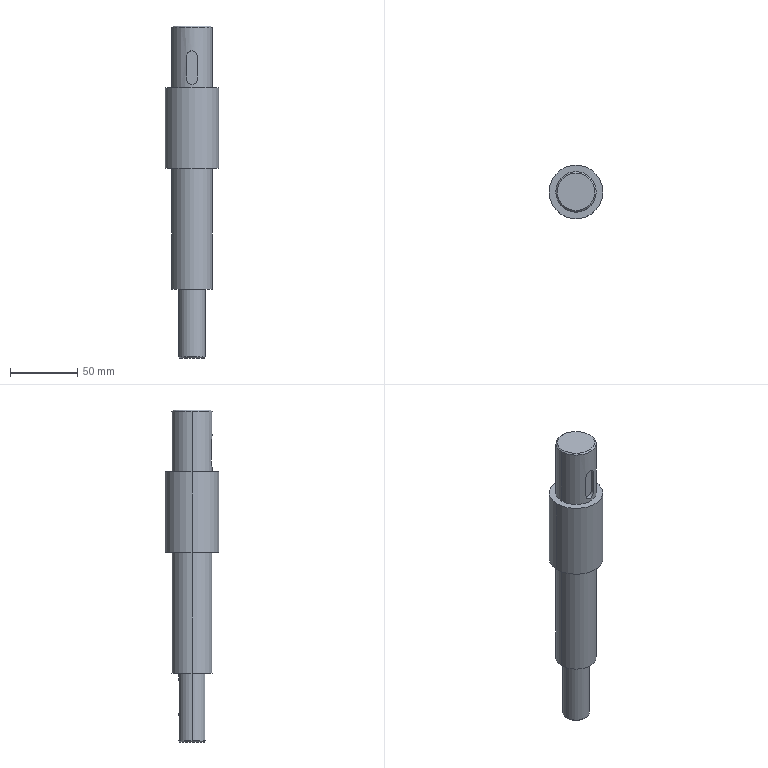Part | SolidWorks | features BaseBody 1 | 1 solid | 27 faces | box 40 x 40 x 247 mm | volume 186572 mm3 | cylinder 12 | plane 11 | cone 4 | commonest cylinder face diameters 30 x4 6 x2 8 x2 20 x2 40 x2
STEP:
#1=CARTESIAN_POINT('',(-9.,0.,0.));
#2=VERTEX_POINT('',#1);
#3=CARTESIAN_POINT('',(9.,0.,0.));
#4=VERTEX_POINT('',#3);
#5=CARTESIAN_POINT('',(0.,0.,0.));
#6=DIRECTION('',(0.,0.,1.));
#7=DIRECTION('',(-1.,0.,0.));
#8=AXIS2_PLACEMENT_3D('',#5,#6,#7);
#9=CIRCLE('',#8,9.);
#10=EDGE_CURVE('',#2,#4,#9,.T.);
#11=ORIENTED_EDGE('',*,*,#10,.T.);
#12=CARTESIAN_POINT('',(10.,0.,1.));
#13=VERTEX_POINT('',#12);
#14=CARTESIAN_POINT('',(9.5,0.,0.5));
#15=DIRECTION('',(0.7071,0.,0.7071));
#16=VECTOR('',#15,1000.);
#17=LINE('',#14,#16);
#18=EDGE_CURVE('',#4,#13,#17,.T.);
#19=ORIENTED_EDGE('',*,*,#18,.T.);
#20=CARTESIAN_POINT('',(-10.,0.,1.));
#21=VERTEX_POINT('',#20);
#22=CARTESIAN_POINT('',(0.,0.,1.));
#23=DIRECTION('',(0.,0.,-1.));
#24=DIRECTION('',(-1.,0.,0.));
#25=AXIS2_PLACEMENT_3D('',#22,#23,#24);
#26=CIRCLE('',#25,10.);
#27=EDGE_CURVE('',#13,#21,#26,.T.);
#28=ORIENTED_EDGE('',*,*,#27,.T.);
#29=CARTESIAN_POINT('',(-9.5,0.,0.5));
#30=DIRECTION('',(-0.7071,0.,0.7071));
#31=VECTOR('',#30,1000.);
#32=LINE('',#29,#31);
#33=EDGE_CURVE('',#2,#21,#32,.T.);
#34=ORIENTED_EDGE('',*,*,#33,.F.);
#35=EDGE_LOOP('',(#11,#19,#28,#34));
#36=FACE_OUTER_BOUND('',#35,.T.);
#37=CARTESIAN_POINT('',(0.,0.,0.5));
#38=DIRECTION('',(0.,0.,1.));
#39=DIRECTION('',(-1.,0.,0.));
#40=AXIS2_PLACEMENT_3D('',#37,#38,#39);
#41=CONICAL_SURFACE('',#40,9.5,0.7854);
#42=ADVANCED_FACE('',(#36),#41,.T.);
#43=CARTESIAN_POINT('',(-3.,9.539,44.5));
#44=VERTEX_POINT('',#43);
#45=CARTESIAN_POINT('',(-3.,9.539,22.5));
#46=VERTEX_POINT('',#45);
#47=CARTESIAN_POINT('',(-3.,9.539,0.));
#48=DIRECTION('',(0.,0.,-1.));
#49=VECTOR('',#48,1000.);
#50=LINE('',#47,#49);
#51=EDGE_CURVE('',#44,#46,#50,.T.);
#52=ORIENTED_EDGE('',*,*,#51,.T.);
#53=CARTESIAN_POINT('',(3.,9.539,22.5));
#54=VERTEX_POINT('',#53);
#55=CARTESIAN_POINT('',(-3.,9.539,22.5));
#56=CARTESIAN_POINT('',(-3.,9.539,22.301));
#57=CARTESIAN_POINT('',(-2.98,9.546,22.105));
#58=CARTESIAN_POINT('',(-2.904,9.569,21.72));
#59=CARTESIAN_POINT('',(-2.845,9.587,21.529));
#60=CARTESIAN_POINT('',(-2.695,9.63,21.167));
#61=CARTESIAN_POINT('',(-2.602,9.656,20.995));
#62=CARTESIAN_POINT('',(-2.385,9.712,20.67));
#63=CARTESIAN_POINT('',(-2.259,9.742,20.517));
#64=CARTESIAN_POINT('',(-1.847,9.832,20.104));
#65=CARTESIAN_POINT('',(-1.515,9.891,19.881));
#66=CARTESIAN_POINT('',(-0.9743,9.954,19.656));
#67=CARTESIAN_POINT('',(-0.7844,9.971,19.598));
#68=CARTESIAN_POINT('',(-0.396,9.994,19.52));
#69=CARTESIAN_POINT('',(-0.1993,10.,19.5));
#70=CARTESIAN_POINT('',(0.1994,10.,19.5));
#71=CARTESIAN_POINT('',(0.3951,9.994,19.52));
#72=CARTESIAN_POINT('',(0.7799,9.971,19.597));
#73=CARTESIAN_POINT('',(0.971,9.954,19.655));
#74=CARTESIAN_POINT('',(1.334,9.912,19.806));
#75=CARTESIAN_POINT('',(1.505,9.887,19.898));
#76=CARTESIAN_POINT('',(1.831,9.832,20.115));
#77=CARTESIAN_POINT('',(1.984,9.802,20.241));
#78=CARTESIAN_POINT('',(2.396,9.713,20.653));
#79=CARTESIAN_POINT('',(2.619,9.652,20.986));
#80=CARTESIAN_POINT('',(2.844,9.587,21.526));
#81=CARTESIAN_POINT('',(2.902,9.57,21.716));
#82=CARTESIAN_POINT('',(2.98,9.546,22.104));
#83=CARTESIAN_POINT('',(3.,9.539,22.301));
#84=CARTESIAN_POINT('',(3.,9.539,22.5));
#85=B_SPLINE_CURVE_WITH_KNOTS('',3,(#55,#56,#57,#58,#59,#60,#61,#62,#63,#64,#65,#66,#67,#68,#69,#70,#71,#72,#73,#74,#75,#76,#77,#78,#79,#80,#81,#82,#83,#84),.UNSPECIFIED.,.F.,.F.,(4,2,2,2,2,2,2,2,2,2,2,2,2,2,4),(0.,0.0005892,0.001178,0.001768,0.002357,0.003535,0.004125,0.004714,0.005303,0.005892,0.006482,0.007071,0.008249,0.008838,0.009428),.UNSPECIFIED.);
#86=EDGE_CURVE('',#46,#54,#85,.T.);
#87=ORIENTED_EDGE('',*,*,#86,.T.);
#88=CARTESIAN_POINT('',(3.,9.539,44.5));
#89=VERTEX_POINT('',#88);
#90=CARTESIAN_POINT('',(3.,9.539,0.));
#91=DIRECTION('',(0.,0.,1.));
#92=VECTOR('',#91,1000.);
#93=LINE('',#90,#92);
#94=EDGE_CURVE('',#54,#89,#93,.T.);
#95=ORIENTED_EDGE('',*,*,#94,.T.);
#96=CARTESIAN_POINT('',(3.,9.539,44.5));
#97=CARTESIAN_POINT('',(3.,9.539,44.699));
#98=CARTESIAN_POINT('',(2.98,9.546,44.895));
#99=CARTESIAN_POINT('',(2.904,9.569,45.28));
#100=CARTESIAN_POINT('',(2.845,9.587,45.471));
#101=CARTESIAN_POINT('',(2.695,9.63,45.833));
#102=CARTESIAN_POINT('',(2.602,9.656,46.005));
#103=CARTESIAN_POINT('',(2.385,9.712,46.33));
#104=CARTESIAN_POINT('',(2.259,9.742,46.483));
#105=CARTESIAN_POINT('',(1.847,9.832,46.896));
#106=CARTESIAN_POINT('',(1.515,9.891,47.119));
#107=CARTESIAN_POINT('',(0.9743,9.954,47.344));
#108=CARTESIAN_POINT('',(0.7844,9.971,47.402));
#109=CARTESIAN_POINT('',(0.396,9.994,47.48));
#110=CARTESIAN_POINT('',(0.1993,10.,47.5));
#111=CARTESIAN_POINT('',(-0.1994,10.,47.5));
#112=CARTESIAN_POINT('',(-0.3951,9.994,47.48));
#113=CARTESIAN_POINT('',(-0.7799,9.971,47.403));
#114=CARTESIAN_POINT('',(-0.971,9.954,47.345));
#115=CARTESIAN_POINT('',(-1.334,9.912,47.194));
#116=CARTESIAN_POINT('',(-1.505,9.887,47.102));
#117=CARTESIAN_POINT('',(-1.831,9.832,46.885));
#118=CARTESIAN_POINT('',(-1.984,9.802,46.759));
#119=CARTESIAN_POINT('',(-2.396,9.713,46.347));
#120=CARTESIAN_POINT('',(-2.619,9.652,46.014));
#121=CARTESIAN_POINT('',(-2.844,9.587,45.474));
#122=CARTESIAN_POINT('',(-2.902,9.57,45.284));
#123=CARTESIAN_POINT('',(-2.98,9.546,44.896));
#124=CARTESIAN_POINT('',(-3.,9.539,44.699));
#125=CARTESIAN_POINT('',(-3.,9.539,44.5));
#126=B_SPLINE_CURVE_WITH_KNOTS('',3,(#96,#97,#98,#99,#100,#101,#102,#103,#104,#105,#106,#107,#108,#109,#110,#111,#112,#113,#114,#115,#116,#117,#118,#119,#120,#121,#122,#123,#124,#125),.UNSPECIFIED.,.F.,.F.,(4,2,2,2,2,2,2,2,2,2,2,2,2,2,4),(0.,0.0005892,0.001178,0.001768,0.002357,0.003535,0.004125,0.004714,0.005303,0.005892,0.006482,0.007071,0.008249,0.008838,0.009428),.UNSPECIFIED.);
#127=EDGE_CURVE('',#89,#44,#126,.T.);
#128=ORIENTED_EDGE('',*,*,#127,.T.);
#129=EDGE_LOOP('',(#52,#87,#95,#128));
#130=FACE_BOUND('',#129,.T.);
#131=CARTESIAN_POINT('',(10.,0.,51.));
#132=VERTEX_POINT('',#131);
#133=CARTESIAN_POINT('',(-10.,0.,51.));
#134=VERTEX_POINT('',#133);
#135=CARTESIAN_POINT('',(0.,0.,51.));
#136=DIRECTION('',(0.,0.,1.));
#137=DIRECTION('',(-1.,0.,0.));
#138=AXIS2_PLACEMENT_3D('',#135,#136,#137);
#139=CIRCLE('',#138,10.);
#140=EDGE_CURVE('',#132,#134,#139,.T.);
#141=ORIENTED_EDGE('',*,*,#140,.F.);
#142=CARTESIAN_POINT('',(10.,0.,0.));
#143=DIRECTION('',(0.,0.,-1.));
#144=VECTOR('',#143,1000.);
#145=LINE('',#142,#144);
#146=EDGE_CURVE('',#132,#13,#145,.T.);
#147=ORIENTED_EDGE('',*,*,#146,.T.);
#148=CARTESIAN_POINT('',(0.,0.,1.));
#149=DIRECTION('',(0.,0.,-1.));
#150=DIRECTION('',(-1.,0.,0.));
#151=AXIS2_PLACEMENT_3D('',#148,#149,#150);
#152=CIRCLE('',#151,10.);
#153=EDGE_CURVE('',#21,#13,#152,.T.);
#154=ORIENTED_EDGE('',*,*,#153,.F.);
#155=CARTESIAN_POINT('',(-10.,0.,0.));
#156=DIRECTION('',(0.,0.,-1.));
#157=VECTOR('',#156,1000.);
#158=LINE('',#155,#157);
#159=EDGE_CURVE('',#134,#21,#158,.T.);
#160=ORIENTED_EDGE('',*,*,#159,.F.);
#161=EDGE_LOOP('',(#141,#147,#154,#160));
#162=FACE_OUTER_BOUND('',#161,.T.);
#163=CARTESIAN_POINT('',(0.,0.,0.));
#164=DIRECTION('',(0.,0.,-1.));
#165=DIRECTION('',(-1.,0.,0.));
#166=AXIS2_PLACEMENT_3D('',#163,#164,#165);
#167=CYLINDRICAL_SURFACE('',#166,10.);
#168=ADVANCED_FACE('',(#130,#162),#167,.T.);
#169=CARTESIAN_POINT('',(-14.,0.,247.));
#170=VERTEX_POINT('',#169);
#171=CARTESIAN_POINT('',(14.,0.,247.));
#172=VERTEX_POINT('',#171);
#173=CARTESIAN_POINT('',(0.,0.,247.));
#174=DIRECTION('',(0.,0.,-1.));
#175=DIRECTION('',(-1.,0.,0.));
#176=AXIS2_PLACEMENT_3D('',#173,#174,#175);
#177=CIRCLE('',#176,14.);
#178=EDGE_CURVE('',#170,#172,#177,.T.);
#179=ORIENTED_EDGE('',*,*,#178,.T.);
#180=CARTESIAN_POINT('',(15.,0.,246.));
#181=VERTEX_POINT('',#180);
#182=CARTESIAN_POINT('',(14.5,0.,246.5));
#183=DIRECTION('',(0.7071,0.,-0.7071));
#184=VECTOR('',#183,1000.);
#185=LINE('',#182,#184);
#186=EDGE_CURVE('',#172,#181,#185,.T.);
#187=ORIENTED_EDGE('',*,*,#186,.T.);
#188=CARTESIAN_POINT('',(-15.,0.,246.));
#189=VERTEX_POINT('',#188);
#190=CARTESIAN_POINT('',(0.,0.,246.));
#191=DIRECTION('',(0.,0.,1.));
#192=DIRECTION('',(-1.,0.,0.));
#193=AXIS2_PLACEMENT_3D('',#190,#191,#192);
#194=CIRCLE('',#193,15.);
#195=EDGE_CURVE('',#181,#189,#194,.T.);
#196=ORIENTED_EDGE('',*,*,#195,.T.);
#197=CARTESIAN_POINT('',(-14.5,0.,246.5));
#198=DIRECTION('',(-0.7071,0.,-0.7071));
#199=VECTOR('',#198,1000.);
#200=LINE('',#197,#199);
#201=EDGE_CURVE('',#170,#189,#200,.T.);
#202=ORIENTED_EDGE('',*,*,#201,.F.);
#203=EDGE_LOOP('',(#179,#187,#196,#202));
#204=FACE_OUTER_BOUND('',#203,.T.);
#205=CARTESIAN_POINT('',(0.,0.,246.5));
#206=DIRECTION('',(0.,0.,-1.));
#207=DIRECTION('',(-1.,0.,0.));
#208=AXIS2_PLACEMENT_3D('',#205,#206,#207);
#209=CONICAL_SURFACE('',#208,14.5,0.7854);
#210=ADVANCED_FACE('',(#204),#209,.T.);
#211=ORIENTED_EDGE('',*,*,#195,.F.);
#212=CARTESIAN_POINT('',(15.,0.,201.));
#213=VERTEX_POINT('',#212);
#214=CARTESIAN_POINT('',(15.,0.,201.));
#215=DIRECTION('',(0.,0.,-1.));
#216=VECTOR('',#215,1000.);
#217=LINE('',#214,#216);
#218=EDGE_CURVE('',#181,#213,#217,.T.);
#219=ORIENTED_EDGE('',*,*,#218,.T.);
#220=CARTESIAN_POINT('',(-15.,0.,201.));
#221=VERTEX_POINT('',#220);
#222=CARTESIAN_POINT('',(0.,0.,201.));
#223=DIRECTION('',(0.,0.,-1.));
#224=DIRECTION('',(-1.,0.,0.));
#225=AXIS2_PLACEMENT_3D('',#222,#223,#224);
#226=CIRCLE('',#225,15.);
#227=EDGE_CURVE('',#221,#213,#226,.T.);
#228=ORIENTED_EDGE('',*,*,#227,.F.);
#229=CARTESIAN_POINT('',(-15.,0.,201.));
#230=DIRECTION('',(0.,0.,-1.));
#231=VECTOR('',#230,1000.);
#232=LINE('',#229,#231);
#233=EDGE_CURVE('',#189,#221,#232,.T.);
#234=ORIENTED_EDGE('',*,*,#233,.F.);
#235=EDGE_LOOP('',(#211,#219,#228,#234));
#236=FACE_OUTER_BOUND('',#235,.T.);
#237=CARTESIAN_POINT('',(0.,0.,201.));
#238=DIRECTION('',(0.,0.,-1.));
#239=DIRECTION('',(-1.,0.,0.));
#240=AXIS2_PLACEMENT_3D('',#237,#238,#239);
#241=CYLINDRICAL_SURFACE('',#240,15.);
#242=ADVANCED_FACE('',(#236),#241,.T.);
#243=CARTESIAN_POINT('',(20.,0.,201.));
#244=VERTEX_POINT('',#243);
#245=CARTESIAN_POINT('',(-20.,0.,201.));
#246=VERTEX_POINT('',#245);
#247=CARTESIAN_POINT('',(0.,0.,201.));
#248=DIRECTION('',(0.,0.,1.));
#249=DIRECTION('',(-1.,0.,0.));
#250=AXIS2_PLACEMENT_3D('',#247,#248,#249);
#251=CIRCLE('',#250,20.);
#252=EDGE_CURVE('',#244,#246,#251,.T.);
#253=ORIENTED_EDGE('',*,*,#252,.F.);
#254=CARTESIAN_POINT('',(20.,0.,141.));
#255=VERTEX_POINT('',#254);
#256=CARTESIAN_POINT('',(20.,0.,141.));
#257=DIRECTION('',(0.,0.,-1.));
#258=VECTOR('',#257,1000.);
#259=LINE('',#256,#258);
#260=EDGE_CURVE('',#244,#255,#259,.T.);
#261=ORIENTED_EDGE('',*,*,#260,.T.);
#262=CARTESIAN_POINT('',(-20.,0.,141.));
#263=VERTEX_POINT('',#262);
#264=CARTESIAN_POINT('',(0.,0.,141.));
#265=DIRECTION('',(0.,0.,-1.));
#266=DIRECTION('',(-1.,0.,0.));
#267=AXIS2_PLACEMENT_3D('',#264,#265,#266);
#268=CIRCLE('',#267,20.);
#269=EDGE_CURVE('',#263,#255,#268,.T.);
#270=ORIENTED_EDGE('',*,*,#269,.F.);
#271=CARTESIAN_POINT('',(-20.,0.,141.));
#272=DIRECTION('',(0.,0.,-1.));
#273=VECTOR('',#272,1000.);
#274=LINE('',#271,#273);
#275=EDGE_CURVE('',#246,#263,#274,.T.);
#276=ORIENTED_EDGE('',*,*,#275,.F.);
#277=EDGE_LOOP('',(#253,#261,#270,#276));
#278=FACE_OUTER_BOUND('',#277,.T.);
#279=CARTESIAN_POINT('',(0.,0.,141.));
#280=DIRECTION('',(0.,0.,-1.));
#281=DIRECTION('',(-1.,0.,0.));
#282=AXIS2_PLACEMENT_3D('',#279,#280,#281);
#283=CYLINDRICAL_SURFACE('',#282,20.);
#284=ADVANCED_FACE('',(#278),#283,.T.);
#285=CARTESIAN_POINT('',(15.,0.,141.));
#286=VERTEX_POINT('',#285);
#287=CARTESIAN_POINT('',(-15.,0.,141.));
#288=VERTEX_POINT('',#287);
#289=CARTESIAN_POINT('',(0.,0.,141.));
#290=DIRECTION('',(0.,0.,1.));
#291=DIRECTION('',(-1.,0.,0.));
#292=AXIS2_PLACEMENT_3D('',#289,#290,#291);
#293=CIRCLE('',#292,15.);
#294=EDGE_CURVE('',#286,#288,#293,.T.);
#295=ORIENTED_EDGE('',*,*,#294,.F.);
#296=CARTESIAN_POINT('',(15.,0.,51.));
#297=VERTEX_POINT('',#296);
#298=CARTESIAN_POINT('',(15.,0.,51.));
#299=DIRECTION('',(0.,0.,-1.));
#300=VECTOR('',#299,1000.);
#301=LINE('',#298,#300);
#302=EDGE_CURVE('',#286,#297,#301,.T.);
#303=ORIENTED_EDGE('',*,*,#302,.T.);
#304=CARTESIAN_POINT('',(-15.,0.,51.));
#305=VERTEX_POINT('',#304);
#306=CARTESIAN_POINT('',(0.,0.,51.));
#307=DIRECTION('',(0.,0.,-1.));
#308=DIRECTION('',(-1.,0.,0.));
#309=AXIS2_PLACEMENT_3D('',#306,#307,#308);
#310=CIRCLE('',#309,15.);
#311=EDGE_CURVE('',#305,#297,#310,.T.);
#312=ORIENTED_EDGE('',*,*,#311,.F.);
#313=CARTESIAN_POINT('',(-15.,0.,51.));
#314=DIRECTION('',(0.,0.,-1.));
#315=VECTOR('',#314,1000.);
#316=LINE('',#313,#315);
#317=EDGE_CURVE('',#288,#305,#316,.T.);
#318=ORIENTED_EDGE('',*,*,#317,.F.);
#319=EDGE_LOOP('',(#295,#303,#312,#318));
#320=FACE_OUTER_BOUND('',#319,.T.);
#321=CARTESIAN_POINT('',(0.,0.,51.));
#322=DIRECTION('',(0.,0.,-1.));
#323=DIRECTION('',(-1.,0.,0.));
#324=AXIS2_PLACEMENT_3D('',#321,#322,#323);
#325=CYLINDRICAL_SURFACE('',#324,15.);
#326=ADVANCED_FACE('',(#320),#325,.T.);
#327=CARTESIAN_POINT('',(-4.,-14.457,207.5));
#328=VERTEX_POINT('',#327);
#329=CARTESIAN_POINT('',(-4.,-14.457,224.5));
#330=VERTEX_POINT('',#329);
#331=CARTESIAN_POINT('',(-4.,-14.457,201.));
#332=DIRECTION('',(0.,0.,1.));
#333=VECTOR('',#332,1000.);
#334=LINE('',#331,#333);
#335=EDGE_CURVE('',#328,#330,#334,.T.);
#336=ORIENTED_EDGE('',*,*,#335,.F.);
#337=CARTESIAN_POINT('',(-4.,-12.,207.5));
#338=VERTEX_POINT('',#337);
#339=CARTESIAN_POINT('',(-4.,-15.,207.5));
#340=DIRECTION('',(0.,1.,0.));
#341=VECTOR('',#340,1000.);
#342=LINE('',#339,#341);
#343=EDGE_CURVE('',#328,#338,#342,.T.);
#344=ORIENTED_EDGE('',*,*,#343,.T.);
#345=CARTESIAN_POINT('',(-4.,-12.,224.5));
#346=VERTEX_POINT('',#345);
#347=CARTESIAN_POINT('',(-4.,-12.,207.5));
#348=DIRECTION('',(0.,0.,1.));
#349=VECTOR('',#348,1000.);
#350=LINE('',#347,#349);
#351=EDGE_CURVE('',#338,#346,#350,.T.);
#352=ORIENTED_EDGE('',*,*,#351,.T.);
#353=CARTESIAN_POINT('',(-4.,-15.,224.5));
#354=DIRECTION('',(0.,1.,0.));
#355=VECTOR('',#354,1000.);
#356=LINE('',#353,#355);
#357=EDGE_CURVE('',#330,#346,#356,.T.);
#358=ORIENTED_EDGE('',*,*,#357,.F.);
#359=EDGE_LOOP('',(#336,#344,#352,#358));
#360=FACE_OUTER_BOUND('',#359,.T.);
#361=CARTESIAN_POINT('',(-4.,-15.,207.5));
#362=DIRECTION('',(-1.,0.,0.));
#363=DIRECTION('',(0.,0.,1.));
#364=AXIS2_PLACEMENT_3D('',#361,#362,#363);
#365=PLANE('',#364);
#366=ADVANCED_FACE('',(#360),#365,.F.);
#367=CARTESIAN_POINT('',(4.,-14.457,224.5));
#368=VERTEX_POINT('',#367);
#369=CARTESIAN_POINT('',(-4.,-14.457,224.5));
#370=CARTESIAN_POINT('',(-4.,-14.457,224.765));
#371=CARTESIAN_POINT('',(-3.974,-14.464,225.026));
#372=CARTESIAN_POINT('',(-3.872,-14.492,225.539));
#373=CARTESIAN_POINT('',(-3.794,-14.513,225.793));
#374=CARTESIAN_POINT('',(-3.593,-14.564,226.277));
#375=CARTESIAN_POINT('',(-3.47,-14.594,226.506));
#376=CARTESIAN_POINT('',(-3.181,-14.66,226.94));
#377=CARTESIAN_POINT('',(-3.013,-14.696,227.144));
#378=CARTESIAN_POINT('',(-2.646,-14.766,227.511));
#379=CARTESIAN_POINT('',(-2.445,-14.801,227.676));
#380=CARTESIAN_POINT('',(-2.009,-14.866,227.969));
#381=CARTESIAN_POINT('',(-1.778,-14.896,228.092));
#382=CARTESIAN_POINT('',(-1.298,-14.946,228.293));
#383=CARTESIAN_POINT('',(-1.045,-14.966,228.37));
#384=CARTESIAN_POINT('',(-0.5274,-14.993,228.474));
#385=CARTESIAN_POINT('',(-0.2653,-15.,228.5));
#386=CARTESIAN_POINT('',(0.2655,-15.,228.5));
#387=CARTESIAN_POINT('',(0.5262,-14.993,228.474));
#388=CARTESIAN_POINT('',(1.039,-14.966,228.372));
#389=CARTESIAN_POINT('',(1.293,-14.946,228.294));
#390=CARTESIAN_POINT('',(1.777,-14.896,228.093));
#391=CARTESIAN_POINT('',(2.006,-14.867,227.97));
#392=CARTESIAN_POINT('',(2.44,-14.802,227.68));
#393=CARTESIAN_POINT('',(2.644,-14.766,227.512));
#394=CARTESIAN_POINT('',(3.011,-14.696,227.146));
#395=CARTESIAN_POINT('',(3.177,-14.661,226.945));
#396=CARTESIAN_POINT('',(3.469,-14.594,226.509));
#397=CARTESIAN_POINT('',(3.592,-14.564,226.278));
#398=CARTESIAN_POINT('',(3.793,-14.513,225.798));
#399=CARTESIAN_POINT('',(3.87,-14.492,225.545));
#400=CARTESIAN_POINT('',(3.974,-14.464,225.027));
#401=CARTESIAN_POINT('',(4.,-14.457,224.765));
#402=CARTESIAN_POINT('',(4.,-14.457,224.5));
#403=B_SPLINE_CURVE_WITH_KNOTS('',3,(#369,#370,#371,#372,#373,#374,#375,#376,#377,#378,#379,#380,#381,#382,#383,#384,#385,#386,#387,#388,#389,#390,#391,#392,#393,#394,#395,#396,#397,#398,#399,#400,#401,#402),.UNSPECIFIED.,.F.,.F.,(4,2,2,2,2,2,2,2,2,2,2,2,2,2,2,2,4),(0.,0.0007847,0.001569,0.002354,0.003139,0.003923,0.004708,0.005493,0.006277,0.007062,0.007847,0.008631,0.009416,0.0102,0.01099,0.01177,0.01255),.UNSPECIFIED.);
#404=EDGE_CURVE('',#330,#368,#403,.T.);
#405=ORIENTED_EDGE('',*,*,#404,.F.);
#406=ORIENTED_EDGE('',*,*,#357,.T.);
#407=CARTESIAN_POINT('',(4.,-12.,224.5));
#408=VERTEX_POINT('',#407);
#409=CARTESIAN_POINT('',(0.,-12.,224.5));
#410=DIRECTION('',(0.,1.,0.));
#411=DIRECTION('',(-1.,0.,0.));
#412=AXIS2_PLACEMENT_3D('',#409,#410,#411);
#413=CIRCLE('',#412,4.);
#414=EDGE_CURVE('',#346,#408,#413,.T.);
#415=ORIENTED_EDGE('',*,*,#414,.T.);
#416=CARTESIAN_POINT('',(4.,-15.,224.5));
#417=DIRECTION('',(0.,1.,0.));
#418=VECTOR('',#417,1000.);
#419=LINE('',#416,#418);
#420=EDGE_CURVE('',#368,#408,#419,.T.);
#421=ORIENTED_EDGE('',*,*,#420,.F.);
#422=EDGE_LOOP('',(#405,#406,#415,#421));
#423=FACE_OUTER_BOUND('',#422,.T.);
#424=CARTESIAN_POINT('',(0.,-15.,224.5));
#425=DIRECTION('',(0.,-1.,0.));
#426=DIRECTION('',(-1.,0.,0.));
#427=AXIS2_PLACEMENT_3D('',#424,#425,#426);
#428=CYLINDRICAL_SURFACE('',#427,4.);
#429=ADVANCED_FACE('',(#423),#428,.F.);
#430=CARTESIAN_POINT('',(4.,-14.457,207.5));
#431=VERTEX_POINT('',#430);
#432=CARTESIAN_POINT('',(4.,-14.457,201.));
#433=DIRECTION('',(0.,0.,-1.));
#434=VECTOR('',#433,1000.);
#435=LINE('',#432,#434);
#436=EDGE_CURVE('',#368,#431,#435,.T.);
#437=ORIENTED_EDGE('',*,*,#436,.F.);
#438=ORIENTED_EDGE('',*,*,#420,.T.);
#439=CARTESIAN_POINT('',(4.,-12.,207.5));
#440=VERTEX_POINT('',#439);
#441=CARTESIAN_POINT('',(4.,-12.,224.5));
#442=DIRECTION('',(0.,0.,-1.));
#443=VECTOR('',#442,1000.);
#444=LINE('',#441,#443);
#445=EDGE_CURVE('',#408,#440,#444,.T.);
#446=ORIENTED_EDGE('',*,*,#445,.T.);
#447=CARTESIAN_POINT('',(4.,-15.,207.5));
#448=DIRECTION('',(0.,1.,0.));
#449=VECTOR('',#448,1000.);
#450=LINE('',#447,#449);
#451=EDGE_CURVE('',#431,#440,#450,.T.);
#452=ORIENTED_EDGE('',*,*,#451,.F.);
#453=EDGE_LOOP('',(#437,#438,#446,#452));
#454=FACE_OUTER_BOUND('',#453,.T.);
#455=CARTESIAN_POINT('',(4.,-15.,224.5));
#456=DIRECTION('',(1.,0.,0.));
#457=DIRECTION('',(0.,0.,-1.));
#458=AXIS2_PLACEMENT_3D('',#455,#456,#457);
#459=PLANE('',#458);
#460=ADVANCED_FACE('',(#454),#459,.F.);
#461=ORIENTED_EDGE('',*,*,#343,.F.);
#462=CARTESIAN_POINT('',(4.,-14.457,207.5));
#463=CARTESIAN_POINT('',(4.,-14.457,207.235));
#464=CARTESIAN_POINT('',(3.974,-14.464,206.974));
#465=CARTESIAN_POINT('',(3.872,-14.492,206.461));
#466=CARTESIAN_POINT('',(3.794,-14.513,206.207));
#467=CARTESIAN_POINT('',(3.593,-14.564,205.723));
#468=CARTESIAN_POINT('',(3.47,-14.594,205.494));
#469=CARTESIAN_POINT('',(3.181,-14.66,205.06));
#470=CARTESIAN_POINT('',(3.013,-14.696,204.856));
#471=CARTESIAN_POINT('',(2.646,-14.766,204.489));
#472=CARTESIAN_POINT('',(2.445,-14.801,204.324));
#473=CARTESIAN_POINT('',(2.009,-14.866,204.031));
#474=CARTESIAN_POINT('',(1.778,-14.896,203.908));
#475=CARTESIAN_POINT('',(1.298,-14.946,203.707));
#476=CARTESIAN_POINT('',(1.045,-14.966,203.63));
#477=CARTESIAN_POINT('',(0.5274,-14.993,203.526));
#478=CARTESIAN_POINT('',(0.2653,-15.,203.5));
#479=CARTESIAN_POINT('',(-0.2655,-15.,203.5));
#480=CARTESIAN_POINT('',(-0.5262,-14.993,203.526));
#481=CARTESIAN_POINT('',(-1.039,-14.966,203.628));
#482=CARTESIAN_POINT('',(-1.293,-14.946,203.706));
#483=CARTESIAN_POINT('',(-1.777,-14.896,203.907));
#484=CARTESIAN_POINT('',(-2.006,-14.867,204.03));
#485=CARTESIAN_POINT('',(-2.44,-14.802,204.32));
#486=CARTESIAN_POINT('',(-2.644,-14.766,204.488));
#487=CARTESIAN_POINT('',(-3.011,-14.696,204.854));
#488=CARTESIAN_POINT('',(-3.177,-14.661,205.055));
#489=CARTESIAN_POINT('',(-3.469,-14.594,205.491));
#490=CARTESIAN_POINT('',(-3.592,-14.564,205.722));
#491=CARTESIAN_POINT('',(-3.793,-14.513,206.202));
#492=CARTESIAN_POINT('',(-3.87,-14.492,206.455));
#493=CARTESIAN_POINT('',(-3.974,-14.464,206.973));
#494=CARTESIAN_POINT('',(-4.,-14.457,207.235));
#495=CARTESIAN_POINT('',(-4.,-14.457,207.5));
#496=B_SPLINE_CURVE_WITH_KNOTS('',3,(#462,#463,#464,#465,#466,#467,#468,#469,#470,#471,#472,#473,#474,#475,#476,#477,#478,#479,#480,#481,#482,#483,#484,#485,#486,#487,#488,#489,#490,#491,#492,#493,#494,#495),.UNSPECIFIED.,.F.,.F.,(4,2,2,2,2,2,2,2,2,2,2,2,2,2,2,2,4),(0.,0.0007847,0.001569,0.002354,0.003139,0.003923,0.004708,0.005493,0.006277,0.007062,0.007847,0.008631,0.009416,0.0102,0.01099,0.01177,0.01255),.UNSPECIFIED.);
#497=EDGE_CURVE('',#431,#328,#496,.T.);
#498=ORIENTED_EDGE('',*,*,#497,.F.);
#499=ORIENTED_EDGE('',*,*,#451,.T.);
#500=CARTESIAN_POINT('',(0.,-12.,207.5));
#501=DIRECTION('',(0.,1.,0.));
#502=DIRECTION('',(1.,0.,0.));
#503=AXIS2_PLACEMENT_3D('',#500,#501,#502);
#504=CIRCLE('',#503,4.);
#505=EDGE_CURVE('',#440,#338,#504,.T.);
#506=ORIENTED_EDGE('',*,*,#505,.T.);
#507=EDGE_LOOP('',(#461,#498,#499,#506));
#508=FACE_OUTER_BOUND('',#507,.T.);
#509=CARTESIAN_POINT('',(0.,-15.,207.5));
#510=DIRECTION('',(0.,-1.,0.));
#511=DIRECTION('',(1.,0.,0.));
#512=AXIS2_PLACEMENT_3D('',#509,#510,#511);
#513=CYLINDRICAL_SURFACE('',#512,4.);
#514=ADVANCED_FACE('',(#508),#513,.F.);
#515=ORIENTED_EDGE('',*,*,#414,.F.);
#516=ORIENTED_EDGE('',*,*,#351,.F.);
#517=ORIENTED_EDGE('',*,*,#505,.F.);
#518=ORIENTED_EDGE('',*,*,#445,.F.);
#519=EDGE_LOOP('',(#515,#516,#517,#518));
#520=FACE_OUTER_BOUND('',#519,.T.);
#521=CARTESIAN_POINT('',(0.,-12.,225.878));
#522=DIRECTION('',(0.,1.,0.));
#523=DIRECTION('',(1.,0.,0.));
#524=AXIS2_PLACEMENT_3D('',#521,#522,#523);
#525=PLANE('',#524);
#526=ADVANCED_FACE('',(#520),#525,.F.);
#527=ORIENTED_EDGE('',*,*,#94,.F.);
#528=CARTESIAN_POINT('',(3.,7.5,22.5));
#529=VERTEX_POINT('',#528);
#530=CARTESIAN_POINT('',(3.,10.,22.5));
#531=DIRECTION('',(0.,-1.,0.));
#532=VECTOR('',#531,1000.);
#533=LINE('',#530,#532);
#534=EDGE_CURVE('',#54,#529,#533,.T.);
#535=ORIENTED_EDGE('',*,*,#534,.T.);
#536=CARTESIAN_POINT('',(3.,7.5,44.5));
#537=VERTEX_POINT('',#536);
#538=CARTESIAN_POINT('',(3.,7.5,44.5));
#539=DIRECTION('',(0.,0.,1.));
#540=VECTOR('',#539,1000.);
#541=LINE('',#538,#540);
#542=EDGE_CURVE('',#529,#537,#541,.T.);
#543=ORIENTED_EDGE('',*,*,#542,.T.);
#544=CARTESIAN_POINT('',(3.,10.,44.5));
#545=DIRECTION('',(0.,-1.,0.));
#546=VECTOR('',#545,1000.);
#547=LINE('',#544,#546);
#548=EDGE_CURVE('',#89,#537,#547,.T.);
#549=ORIENTED_EDGE('',*,*,#548,.F.);
#550=EDGE_LOOP('',(#527,#535,#543,#549));
#551=FACE_OUTER_BOUND('',#550,.T.);
#552=CARTESIAN_POINT('',(3.,10.,22.5));
#553=DIRECTION('',(1.,0.,0.));
#554=DIRECTION('',(0.,1.,0.));
#555=AXIS2_PLACEMENT_3D('',#552,#553,#554);
#556=PLANE('',#555);
#557=ADVANCED_FACE('',(#551),#556,.F.);
#558=ORIENTED_EDGE('',*,*,#127,.F.);
#559=ORIENTED_EDGE('',*,*,#548,.T.);
#560=CARTESIAN_POINT('',(-3.,7.5,44.5));
#561=VERTEX_POINT('',#560);
#562=CARTESIAN_POINT('',(0.,7.5,44.5));
#563=DIRECTION('',(0.,-1.,0.));
#564=DIRECTION('',(-1.,0.,0.));
#565=AXIS2_PLACEMENT_3D('',#562,#563,#564);
#566=CIRCLE('',#565,3.);
#567=EDGE_CURVE('',#537,#561,#566,.T.);
#568=ORIENTED_EDGE('',*,*,#567,.T.);
#569=CARTESIAN_POINT('',(-3.,10.,44.5));
#570=DIRECTION('',(0.,-1.,0.));
#571=VECTOR('',#570,1000.);
#572=LINE('',#569,#571);
#573=EDGE_CURVE('',#44,#561,#572,.T.);
#574=ORIENTED_EDGE('',*,*,#573,.F.);
#575=EDGE_LOOP('',(#558,#559,#568,#574));
#576=FACE_OUTER_BOUND('',#575,.T.);
#577=CARTESIAN_POINT('',(0.,10.,44.5));
#578=DIRECTION('',(0.,1.,0.));
#579=DIRECTION('',(-1.,0.,0.));
#580=AXIS2_PLACEMENT_3D('',#577,#578,#579);
#581=CYLINDRICAL_SURFACE('',#580,3.);
#582=ADVANCED_FACE('',(#576),#581,.F.);
#583=ORIENTED_EDGE('',*,*,#51,.F.);
#584=ORIENTED_EDGE('',*,*,#573,.T.);
#585=CARTESIAN_POINT('',(-3.,7.5,22.5));
#586=VERTEX_POINT('',#585);
#587=CARTESIAN_POINT('',(-3.,7.5,22.5));
#588=DIRECTION('',(0.,0.,-1.));
#589=VECTOR('',#588,1000.);
#590=LINE('',#587,#589);
#591=EDGE_CURVE('',#561,#586,#590,.T.);
#592=ORIENTED_EDGE('',*,*,#591,.T.);
#593=CARTESIAN_POINT('',(-3.,10.,22.5));
#594=DIRECTION('',(0.,-1.,0.));
#595=VECTOR('',#594,1000.);
#596=LINE('',#593,#595);
#597=EDGE_CURVE('',#46,#586,#596,.T.);
#598=ORIENTED_EDGE('',*,*,#597,.F.);
#599=EDGE_LOOP('',(#583,#584,#592,#598));
#600=FACE_OUTER_BOUND('',#599,.T.);
#601=CARTESIAN_POINT('',(-3.,10.,44.5));
#602=DIRECTION('',(-1.,0.,0.));
#603=DIRECTION('',(0.,1.,0.));
#604=AXIS2_PLACEMENT_3D('',#601,#602,#603);
#605=PLANE('',#604);
#606=ADVANCED_FACE('',(#600),#605,.F.);
#607=ORIENTED_EDGE('',*,*,#534,.F.);
#608=ORIENTED_EDGE('',*,*,#86,.F.);
#609=ORIENTED_EDGE('',*,*,#597,.T.);
#610=CARTESIAN_POINT('',(0.,7.5,22.5));
#611=DIRECTION('',(0.,-1.,0.));
#612=DIRECTION('',(1.,0.,0.));
#613=AXIS2_PLACEMENT_3D('',#610,#611,#612);
#614=CIRCLE('',#613,3.);
#615=EDGE_CURVE('',#586,#529,#614,.T.);
#616=ORIENTED_EDGE('',*,*,#615,.T.);
#617=EDGE_LOOP('',(#607,#608,#609,#616));
#618=FACE_OUTER_BOUND('',#617,.T.);
#619=CARTESIAN_POINT('',(0.,10.,22.5));
#620=DIRECTION('',(0.,1.,0.));
#621=DIRECTION('',(1.,0.,0.));
#622=AXIS2_PLACEMENT_3D('',#619,#620,#621);
#623=CYLINDRICAL_SURFACE('',#622,3.);
#624=ADVANCED_FACE('',(#618),#623,.F.);
#625=ORIENTED_EDGE('',*,*,#567,.F.);
#626=ORIENTED_EDGE('',*,*,#542,.F.);
#627=ORIENTED_EDGE('',*,*,#615,.F.);
#628=ORIENTED_EDGE('',*,*,#591,.F.);
#629=EDGE_LOOP('',(#625,#626,#627,#628));
#630=FACE_OUTER_BOUND('',#629,.T.);
#631=CARTESIAN_POINT('',(0.,7.5,45.533));
#632=DIRECTION('',(0.,1.,0.));
#633=DIRECTION('',(1.,0.,0.));
#634=AXIS2_PLACEMENT_3D('',#631,#632,#633);
#635=PLANE('',#634);
#636=ADVANCED_FACE('',(#630),#635,.T.);
#637=ORIENTED_EDGE('',*,*,#10,.F.);
#638=CARTESIAN_POINT('',(0.,0.,0.));
#639=DIRECTION('',(0.,0.,1.));
#640=DIRECTION('',(-1.,0.,0.));
#641=AXIS2_PLACEMENT_3D('',#638,#639,#640);
#642=CIRCLE('',#641,9.);
#643=EDGE_CURVE('',#4,#2,#642,.T.);
#644=ORIENTED_EDGE('',*,*,#643,.F.);
#645=EDGE_LOOP('',(#637,#644));
#646=FACE_OUTER_BOUND('',#645,.T.);
#647=CARTESIAN_POINT('',(0.,0.,0.));
#648=DIRECTION('',(0.,0.,1.));
#649=DIRECTION('',(1.,0.,0.));
#650=AXIS2_PLACEMENT_3D('',#647,#648,#649);
#651=PLANE('',#650);
#652=ADVANCED_FACE('',(#646),#651,.F.);
#653=ORIENTED_EDGE('',*,*,#178,.F.);
#654=CARTESIAN_POINT('',(0.,0.,247.));
#655=DIRECTION('',(0.,0.,-1.));
#656=DIRECTION('',(-1.,0.,0.));
#657=AXIS2_PLACEMENT_3D('',#654,#655,#656);
#658=CIRCLE('',#657,14.);
#659=EDGE_CURVE('',#172,#170,#658,.T.);
#660=ORIENTED_EDGE('',*,*,#659,.F.);
#661=EDGE_LOOP('',(#653,#660));
#662=FACE_OUTER_BOUND('',#661,.T.);
#663=CARTESIAN_POINT('',(0.,0.,247.));
#664=DIRECTION('',(0.,0.,1.));
#665=DIRECTION('',(1.,0.,0.));
#666=AXIS2_PLACEMENT_3D('',#663,#664,#665);
#667=PLANE('',#666);
#668=ADVANCED_FACE('',(#662),#667,.T.);
#669=CARTESIAN_POINT('',(0.,0.,141.));
#670=DIRECTION('',(0.,0.,1.));
#671=DIRECTION('',(-1.,0.,0.));
#672=AXIS2_PLACEMENT_3D('',#669,#670,#671);
#673=CIRCLE('',#672,15.);
#674=EDGE_CURVE('',#288,#286,#673,.T.);
#675=ORIENTED_EDGE('',*,*,#674,.T.);
#676=ORIENTED_EDGE('',*,*,#294,.T.);
#677=EDGE_LOOP('',(#675,#676));
#678=FACE_BOUND('',#677,.T.);
#679=ORIENTED_EDGE('',*,*,#269,.T.);
#680=CARTESIAN_POINT('',(0.,0.,141.));
#681=DIRECTION('',(0.,0.,-1.));
#682=DIRECTION('',(-1.,0.,0.));
#683=AXIS2_PLACEMENT_3D('',#680,#681,#682);
#684=CIRCLE('',#683,20.);
#685=EDGE_CURVE('',#255,#263,#684,.T.);
#686=ORIENTED_EDGE('',*,*,#685,.T.);
#687=EDGE_LOOP('',(#679,#686));
#688=FACE_OUTER_BOUND('',#687,.T.);
#689=CARTESIAN_POINT('',(0.,0.,141.));
#690=DIRECTION('',(0.,0.,1.));
#691=DIRECTION('',(1.,0.,0.));
#692=AXIS2_PLACEMENT_3D('',#689,#690,#691);
#693=PLANE('',#692);
#694=ADVANCED_FACE('',(#678,#688),#693,.F.);
#695=ORIENTED_EDGE('',*,*,#227,.T.);
#696=CARTESIAN_POINT('',(0.,0.,201.));
#697=DIRECTION('',(0.,0.,-1.));
#698=DIRECTION('',(-1.,0.,0.));
#699=AXIS2_PLACEMENT_3D('',#696,#697,#698);
#700=CIRCLE('',#699,15.);
#701=EDGE_CURVE('',#213,#221,#700,.T.);
#702=ORIENTED_EDGE('',*,*,#701,.T.);
#703=EDGE_LOOP('',(#695,#702));
#704=FACE_BOUND('',#703,.T.);
#705=CARTESIAN_POINT('',(0.,0.,201.));
#706=DIRECTION('',(0.,0.,1.));
#707=DIRECTION('',(-1.,0.,0.));
#708=AXIS2_PLACEMENT_3D('',#705,#706,#707);
#709=CIRCLE('',#708,20.);
#710=EDGE_CURVE('',#246,#244,#709,.T.);
#711=ORIENTED_EDGE('',*,*,#710,.T.);
#712=ORIENTED_EDGE('',*,*,#252,.T.);
#713=EDGE_LOOP('',(#711,#712));
#714=FACE_OUTER_BOUND('',#713,.T.);
#715=CARTESIAN_POINT('',(0.,0.,201.));
#716=DIRECTION('',(0.,0.,1.));
#717=DIRECTION('',(1.,0.,0.));
#718=AXIS2_PLACEMENT_3D('',#715,#716,#717);
#719=PLANE('',#718);
#720=ADVANCED_FACE('',(#704,#714),#719,.T.);
#721=CARTESIAN_POINT('',(0.,0.,51.));
#722=DIRECTION('',(0.,0.,1.));
#723=DIRECTION('',(-1.,0.,0.));
#724=AXIS2_PLACEMENT_3D('',#721,#722,#723);
#725=CIRCLE('',#724,10.);
#726=EDGE_CURVE('',#134,#132,#725,.T.);
#727=ORIENTED_EDGE('',*,*,#726,.T.);
#728=ORIENTED_EDGE('',*,*,#140,.T.);
#729=EDGE_LOOP('',(#727,#728));
#730=FACE_BOUND('',#729,.T.);
#731=ORIENTED_EDGE('',*,*,#311,.T.);
#732=CARTESIAN_POINT('',(0.,0.,51.));
#733=DIRECTION('',(0.,0.,-1.));
#734=DIRECTION('',(-1.,0.,0.));
#735=AXIS2_PLACEMENT_3D('',#732,#733,#734);
#736=CIRCLE('',#735,15.);
#737=EDGE_CURVE('',#297,#305,#736,.T.);
#738=ORIENTED_EDGE('',*,*,#737,.T.);
#739=EDGE_LOOP('',(#731,#738));
#740=FACE_OUTER_BOUND('',#739,.T.);
#741=CARTESIAN_POINT('',(0.,0.,51.));
#742=DIRECTION('',(0.,0.,1.));
#743=DIRECTION('',(1.,0.,0.));
#744=AXIS2_PLACEMENT_3D('',#741,#742,#743);
#745=PLANE('',#744);
#746=ADVANCED_FACE('',(#730,#740),#745,.F.);
#747=ORIENTED_EDGE('',*,*,#302,.F.);
#748=ORIENTED_EDGE('',*,*,#674,.F.);
#749=ORIENTED_EDGE('',*,*,#317,.T.);
#750=ORIENTED_EDGE('',*,*,#737,.F.);
#751=EDGE_LOOP('',(#747,#748,#749,#750));
#752=FACE_OUTER_BOUND('',#751,.T.);
#753=CARTESIAN_POINT('',(0.,0.,51.));
#754=DIRECTION('',(0.,0.,-1.));
#755=DIRECTION('',(-1.,0.,0.));
#756=AXIS2_PLACEMENT_3D('',#753,#754,#755);
#757=CYLINDRICAL_SURFACE('',#756,15.);
#758=ADVANCED_FACE('',(#752),#757,.T.);
#759=ORIENTED_EDGE('',*,*,#260,.F.);
#760=ORIENTED_EDGE('',*,*,#710,.F.);
#761=ORIENTED_EDGE('',*,*,#275,.T.);
#762=ORIENTED_EDGE('',*,*,#685,.F.);
#763=EDGE_LOOP('',(#759,#760,#761,#762));
#764=FACE_OUTER_BOUND('',#763,.T.);
#765=CARTESIAN_POINT('',(0.,0.,141.));
#766=DIRECTION('',(0.,0.,-1.));
#767=DIRECTION('',(-1.,0.,0.));
#768=AXIS2_PLACEMENT_3D('',#765,#766,#767);
#769=CYLINDRICAL_SURFACE('',#768,20.);
#770=ADVANCED_FACE('',(#764),#769,.T.);
#771=ORIENTED_EDGE('',*,*,#218,.F.);
#772=CARTESIAN_POINT('',(0.,0.,246.));
#773=DIRECTION('',(0.,0.,1.));
#774=DIRECTION('',(-1.,0.,0.));
#775=AXIS2_PLACEMENT_3D('',#772,#773,#774);
#776=CIRCLE('',#775,15.);
#777=EDGE_CURVE('',#189,#181,#776,.T.);
#778=ORIENTED_EDGE('',*,*,#777,.F.);
#779=ORIENTED_EDGE('',*,*,#233,.T.);
#780=ORIENTED_EDGE('',*,*,#701,.F.);
#781=EDGE_LOOP('',(#771,#778,#779,#780));
#782=FACE_OUTER_BOUND('',#781,.T.);
#783=ORIENTED_EDGE('',*,*,#436,.T.);
#784=ORIENTED_EDGE('',*,*,#497,.T.);
#785=ORIENTED_EDGE('',*,*,#335,.T.);
#786=ORIENTED_EDGE('',*,*,#404,.T.);
#787=EDGE_LOOP('',(#783,#784,#785,#786));
#788=FACE_BOUND('',#787,.T.);
#789=CARTESIAN_POINT('',(0.,0.,201.));
#790=DIRECTION('',(0.,0.,-1.));
#791=DIRECTION('',(-1.,0.,0.));
#792=AXIS2_PLACEMENT_3D('',#789,#790,#791);
#793=CYLINDRICAL_SURFACE('',#792,15.);
#794=ADVANCED_FACE('',(#782,#788),#793,.T.);
#795=ORIENTED_EDGE('',*,*,#186,.F.);
#796=ORIENTED_EDGE('',*,*,#659,.T.);
#797=ORIENTED_EDGE('',*,*,#201,.T.);
#798=ORIENTED_EDGE('',*,*,#777,.T.);
#799=EDGE_LOOP('',(#795,#796,#797,#798));
#800=FACE_OUTER_BOUND('',#799,.T.);
#801=CARTESIAN_POINT('',(0.,0.,246.5));
#802=DIRECTION('',(0.,0.,-1.));
#803=DIRECTION('',(-1.,0.,0.));
#804=AXIS2_PLACEMENT_3D('',#801,#802,#803);
#805=CONICAL_SURFACE('',#804,14.5,0.7854);
#806=ADVANCED_FACE('',(#800),#805,.T.);
#807=ORIENTED_EDGE('',*,*,#146,.F.);
#808=ORIENTED_EDGE('',*,*,#726,.F.);
#809=ORIENTED_EDGE('',*,*,#159,.T.);
#810=ORIENTED_EDGE('',*,*,#27,.F.);
#811=EDGE_LOOP('',(#807,#808,#809,#810));
#812=FACE_OUTER_BOUND('',#811,.T.);
#813=CARTESIAN_POINT('',(0.,0.,0.));
#814=DIRECTION('',(0.,0.,-1.));
#815=DIRECTION('',(-1.,0.,0.));
#816=AXIS2_PLACEMENT_3D('',#813,#814,#815);
#817=CYLINDRICAL_SURFACE('',#816,10.);
#818=ADVANCED_FACE('',(#812),#817,.T.);
#819=ORIENTED_EDGE('',*,*,#18,.F.);
#820=ORIENTED_EDGE('',*,*,#643,.T.);
#821=ORIENTED_EDGE('',*,*,#33,.T.);
#822=ORIENTED_EDGE('',*,*,#153,.T.);
#823=EDGE_LOOP('',(#819,#820,#821,#822));
#824=FACE_OUTER_BOUND('',#823,.T.);
#825=CARTESIAN_POINT('',(0.,0.,0.5));
#826=DIRECTION('',(0.,0.,1.));
#827=DIRECTION('',(-1.,0.,0.));
#828=AXIS2_PLACEMENT_3D('',#825,#826,#827);
#829=CONICAL_SURFACE('',#828,9.5,0.7854);
#830=ADVANCED_FACE('',(#824),#829,.T.);
#831=CLOSED_SHELL('',(#42,#168,#210,#242,#284,#326,#366,#429,#460,#514,#526,#557,#582,#606,#624,#636,#652,#668,#694,#720,#746,#758,#770,#794,#806,#818,#830));
#832=MANIFOLD_SOLID_BREP('',#831);
#833=CARTESIAN_POINT('',(0.,0.,0.));
#834=DIRECTION('',(0.,0.,1.));
#835=DIRECTION('',(1.,0.,0.));
#836=AXIS2_PLACEMENT_3D('',#833,#834,#835);
#837=(LENGTH_UNIT()NAMED_UNIT(*)SI_UNIT(.MILLI.,.METRE.));
#838=UNCERTAINTY_MEASURE_WITH_UNIT(LENGTH_MEASURE(0.00001),#837,'','');
#839=(NAMED_UNIT(*)PLANE_ANGLE_UNIT()SI_UNIT($,.RADIAN.));
#840=(NAMED_UNIT(*)SI_UNIT($,.STERADIAN.)SOLID_ANGLE_UNIT());
#841=(GEOMETRIC_REPRESENTATION_CONTEXT(3)GLOBAL_UNCERTAINTY_ASSIGNED_CONTEXT((#838))GLOBAL_UNIT_ASSIGNED_CONTEXT((#837,#839,#840))REPRESENTATION_CONTEXT('',''));
#842=ADVANCED_BREP_SHAPE_REPRESENTATION('',(#832,#836),#841);